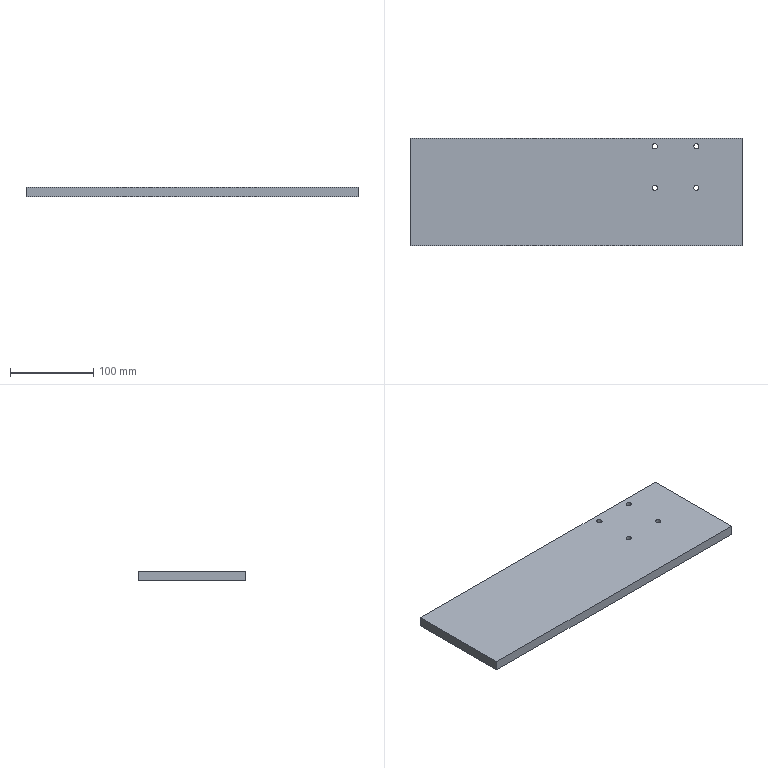Part | SolidWorks | features BaseBody 1 | 1 solid | 14 faces | box 400 x 130 x 12 mm | volume 622504 mm3 | cylinder 8 | plane 6 | commonest cylinder face diameters 6.3 x8
STEP:
#1=CARTESIAN_POINT('',(141.85,55.,-6.));
#2=VERTEX_POINT('',#1);
#3=CARTESIAN_POINT('',(148.15,55.,-6.));
#4=VERTEX_POINT('',#3);
#5=CARTESIAN_POINT('',(145.,55.,-6.));
#6=DIRECTION('',(0.,0.,1.));
#7=DIRECTION('',(1.,0.,0.));
#8=AXIS2_PLACEMENT_3D('',#5,#6,#7);
#9=CIRCLE('',#8,3.15);
#10=EDGE_CURVE('',#2,#4,#9,.T.);
#11=ORIENTED_EDGE('',*,*,#10,.F.);
#12=CARTESIAN_POINT('',(141.85,55.,6.));
#13=VERTEX_POINT('',#12);
#14=CARTESIAN_POINT('',(141.85,55.,-14.2));
#15=DIRECTION('',(0.,0.,1.));
#16=VECTOR('',#15,1000.);
#17=LINE('',#14,#16);
#18=EDGE_CURVE('',#2,#13,#17,.T.);
#19=ORIENTED_EDGE('',*,*,#18,.T.);
#20=CARTESIAN_POINT('',(148.15,55.,6.));
#21=VERTEX_POINT('',#20);
#22=CARTESIAN_POINT('',(145.,55.,6.));
#23=DIRECTION('',(0.,0.,-1.));
#24=DIRECTION('',(1.,0.,0.));
#25=AXIS2_PLACEMENT_3D('',#22,#23,#24);
#26=CIRCLE('',#25,3.15);
#27=EDGE_CURVE('',#21,#13,#26,.T.);
#28=ORIENTED_EDGE('',*,*,#27,.F.);
#29=CARTESIAN_POINT('',(148.15,55.,-14.2));
#30=DIRECTION('',(0.,0.,1.));
#31=VECTOR('',#30,1000.);
#32=LINE('',#29,#31);
#33=EDGE_CURVE('',#4,#21,#32,.T.);
#34=ORIENTED_EDGE('',*,*,#33,.F.);
#35=EDGE_LOOP('',(#11,#19,#28,#34));
#36=FACE_OUTER_BOUND('',#35,.T.);
#37=CARTESIAN_POINT('',(145.,55.,-14.2));
#38=DIRECTION('',(0.,0.,1.));
#39=DIRECTION('',(1.,0.,0.));
#40=AXIS2_PLACEMENT_3D('',#37,#38,#39);
#41=CYLINDRICAL_SURFACE('',#40,3.15);
#42=ADVANCED_FACE('',(#36),#41,.F.);
#43=CARTESIAN_POINT('',(91.85,55.,-6.));
#44=VERTEX_POINT('',#43);
#45=CARTESIAN_POINT('',(98.15,55.,-6.));
#46=VERTEX_POINT('',#45);
#47=CARTESIAN_POINT('',(95.,55.,-6.));
#48=DIRECTION('',(0.,0.,1.));
#49=DIRECTION('',(1.,0.,0.));
#50=AXIS2_PLACEMENT_3D('',#47,#48,#49);
#51=CIRCLE('',#50,3.15);
#52=EDGE_CURVE('',#44,#46,#51,.T.);
#53=ORIENTED_EDGE('',*,*,#52,.F.);
#54=CARTESIAN_POINT('',(91.85,55.,6.));
#55=VERTEX_POINT('',#54);
#56=CARTESIAN_POINT('',(91.85,55.,-14.2));
#57=DIRECTION('',(0.,0.,1.));
#58=VECTOR('',#57,1000.);
#59=LINE('',#56,#58);
#60=EDGE_CURVE('',#44,#55,#59,.T.);
#61=ORIENTED_EDGE('',*,*,#60,.T.);
#62=CARTESIAN_POINT('',(98.15,55.,6.));
#63=VERTEX_POINT('',#62);
#64=CARTESIAN_POINT('',(95.,55.,6.));
#65=DIRECTION('',(0.,0.,-1.));
#66=DIRECTION('',(1.,0.,0.));
#67=AXIS2_PLACEMENT_3D('',#64,#65,#66);
#68=CIRCLE('',#67,3.15);
#69=EDGE_CURVE('',#63,#55,#68,.T.);
#70=ORIENTED_EDGE('',*,*,#69,.F.);
#71=CARTESIAN_POINT('',(98.15,55.,-14.2));
#72=DIRECTION('',(0.,0.,1.));
#73=VECTOR('',#72,1000.);
#74=LINE('',#71,#73);
#75=EDGE_CURVE('',#46,#63,#74,.T.);
#76=ORIENTED_EDGE('',*,*,#75,.F.);
#77=EDGE_LOOP('',(#53,#61,#70,#76));
#78=FACE_OUTER_BOUND('',#77,.T.);
#79=CARTESIAN_POINT('',(95.,55.,-14.2));
#80=DIRECTION('',(0.,0.,1.));
#81=DIRECTION('',(1.,0.,0.));
#82=AXIS2_PLACEMENT_3D('',#79,#80,#81);
#83=CYLINDRICAL_SURFACE('',#82,3.15);
#84=ADVANCED_FACE('',(#78),#83,.F.);
#85=CARTESIAN_POINT('',(141.85,5.,-6.));
#86=VERTEX_POINT('',#85);
#87=CARTESIAN_POINT('',(148.15,5.,-6.));
#88=VERTEX_POINT('',#87);
#89=CARTESIAN_POINT('',(145.,5.,-6.));
#90=DIRECTION('',(0.,0.,1.));
#91=DIRECTION('',(1.,0.,0.));
#92=AXIS2_PLACEMENT_3D('',#89,#90,#91);
#93=CIRCLE('',#92,3.15);
#94=EDGE_CURVE('',#86,#88,#93,.T.);
#95=ORIENTED_EDGE('',*,*,#94,.F.);
#96=CARTESIAN_POINT('',(141.85,5.,6.));
#97=VERTEX_POINT('',#96);
#98=CARTESIAN_POINT('',(141.85,5.,-14.2));
#99=DIRECTION('',(0.,0.,1.));
#100=VECTOR('',#99,1000.);
#101=LINE('',#98,#100);
#102=EDGE_CURVE('',#86,#97,#101,.T.);
#103=ORIENTED_EDGE('',*,*,#102,.T.);
#104=CARTESIAN_POINT('',(148.15,5.,6.));
#105=VERTEX_POINT('',#104);
#106=CARTESIAN_POINT('',(145.,5.,6.));
#107=DIRECTION('',(0.,0.,-1.));
#108=DIRECTION('',(1.,0.,0.));
#109=AXIS2_PLACEMENT_3D('',#106,#107,#108);
#110=CIRCLE('',#109,3.15);
#111=EDGE_CURVE('',#105,#97,#110,.T.);
#112=ORIENTED_EDGE('',*,*,#111,.F.);
#113=CARTESIAN_POINT('',(148.15,5.,-14.2));
#114=DIRECTION('',(0.,0.,1.));
#115=VECTOR('',#114,1000.);
#116=LINE('',#113,#115);
#117=EDGE_CURVE('',#88,#105,#116,.T.);
#118=ORIENTED_EDGE('',*,*,#117,.F.);
#119=EDGE_LOOP('',(#95,#103,#112,#118));
#120=FACE_OUTER_BOUND('',#119,.T.);
#121=CARTESIAN_POINT('',(145.,5.,-14.2));
#122=DIRECTION('',(0.,0.,1.));
#123=DIRECTION('',(1.,0.,0.));
#124=AXIS2_PLACEMENT_3D('',#121,#122,#123);
#125=CYLINDRICAL_SURFACE('',#124,3.15);
#126=ADVANCED_FACE('',(#120),#125,.F.);
#127=CARTESIAN_POINT('',(91.85,5.,-6.));
#128=VERTEX_POINT('',#127);
#129=CARTESIAN_POINT('',(98.15,5.,-6.));
#130=VERTEX_POINT('',#129);
#131=CARTESIAN_POINT('',(95.,5.,-6.));
#132=DIRECTION('',(0.,0.,1.));
#133=DIRECTION('',(1.,0.,0.));
#134=AXIS2_PLACEMENT_3D('',#131,#132,#133);
#135=CIRCLE('',#134,3.15);
#136=EDGE_CURVE('',#128,#130,#135,.T.);
#137=ORIENTED_EDGE('',*,*,#136,.F.);
#138=CARTESIAN_POINT('',(91.85,5.,6.));
#139=VERTEX_POINT('',#138);
#140=CARTESIAN_POINT('',(91.85,5.,-14.2));
#141=DIRECTION('',(0.,0.,1.));
#142=VECTOR('',#141,1000.);
#143=LINE('',#140,#142);
#144=EDGE_CURVE('',#128,#139,#143,.T.);
#145=ORIENTED_EDGE('',*,*,#144,.T.);
#146=CARTESIAN_POINT('',(98.15,5.,6.));
#147=VERTEX_POINT('',#146);
#148=CARTESIAN_POINT('',(95.,5.,6.));
#149=DIRECTION('',(0.,0.,-1.));
#150=DIRECTION('',(1.,0.,0.));
#151=AXIS2_PLACEMENT_3D('',#148,#149,#150);
#152=CIRCLE('',#151,3.15);
#153=EDGE_CURVE('',#147,#139,#152,.T.);
#154=ORIENTED_EDGE('',*,*,#153,.F.);
#155=CARTESIAN_POINT('',(98.15,5.,-14.2));
#156=DIRECTION('',(0.,0.,1.));
#157=VECTOR('',#156,1000.);
#158=LINE('',#155,#157);
#159=EDGE_CURVE('',#130,#147,#158,.T.);
#160=ORIENTED_EDGE('',*,*,#159,.F.);
#161=EDGE_LOOP('',(#137,#145,#154,#160));
#162=FACE_OUTER_BOUND('',#161,.T.);
#163=CARTESIAN_POINT('',(95.,5.,-14.2));
#164=DIRECTION('',(0.,0.,1.));
#165=DIRECTION('',(1.,0.,0.));
#166=AXIS2_PLACEMENT_3D('',#163,#164,#165);
#167=CYLINDRICAL_SURFACE('',#166,3.15);
#168=ADVANCED_FACE('',(#162),#167,.F.);
#169=ORIENTED_EDGE('',*,*,#27,.T.);
#170=CARTESIAN_POINT('',(145.,55.,6.));
#171=DIRECTION('',(0.,0.,-1.));
#172=DIRECTION('',(1.,0.,0.));
#173=AXIS2_PLACEMENT_3D('',#170,#171,#172);
#174=CIRCLE('',#173,3.15);
#175=EDGE_CURVE('',#13,#21,#174,.T.);
#176=ORIENTED_EDGE('',*,*,#175,.T.);
#177=EDGE_LOOP('',(#169,#176));
#178=FACE_BOUND('',#177,.T.);
#179=ORIENTED_EDGE('',*,*,#69,.T.);
#180=CARTESIAN_POINT('',(95.,55.,6.));
#181=DIRECTION('',(0.,0.,-1.));
#182=DIRECTION('',(1.,0.,0.));
#183=AXIS2_PLACEMENT_3D('',#180,#181,#182);
#184=CIRCLE('',#183,3.15);
#185=EDGE_CURVE('',#55,#63,#184,.T.);
#186=ORIENTED_EDGE('',*,*,#185,.T.);
#187=EDGE_LOOP('',(#179,#186));
#188=FACE_BOUND('',#187,.T.);
#189=ORIENTED_EDGE('',*,*,#111,.T.);
#190=CARTESIAN_POINT('',(145.,5.,6.));
#191=DIRECTION('',(0.,0.,-1.));
#192=DIRECTION('',(1.,0.,0.));
#193=AXIS2_PLACEMENT_3D('',#190,#191,#192);
#194=CIRCLE('',#193,3.15);
#195=EDGE_CURVE('',#97,#105,#194,.T.);
#196=ORIENTED_EDGE('',*,*,#195,.T.);
#197=EDGE_LOOP('',(#189,#196));
#198=FACE_BOUND('',#197,.T.);
#199=ORIENTED_EDGE('',*,*,#153,.T.);
#200=CARTESIAN_POINT('',(95.,5.,6.));
#201=DIRECTION('',(0.,0.,-1.));
#202=DIRECTION('',(1.,0.,0.));
#203=AXIS2_PLACEMENT_3D('',#200,#201,#202);
#204=CIRCLE('',#203,3.15);
#205=EDGE_CURVE('',#139,#147,#204,.T.);
#206=ORIENTED_EDGE('',*,*,#205,.T.);
#207=EDGE_LOOP('',(#199,#206));
#208=FACE_BOUND('',#207,.T.);
#209=CARTESIAN_POINT('',(200.,-65.,6.));
#210=VERTEX_POINT('',#209);
#211=CARTESIAN_POINT('',(200.,65.,6.));
#212=VERTEX_POINT('',#211);
#213=CARTESIAN_POINT('',(200.,-65.,6.));
#214=DIRECTION('',(0.,1.,0.));
#215=VECTOR('',#214,1000.);
#216=LINE('',#213,#215);
#217=EDGE_CURVE('',#210,#212,#216,.T.);
#218=ORIENTED_EDGE('',*,*,#217,.T.);
#219=CARTESIAN_POINT('',(-200.,65.,6.));
#220=VERTEX_POINT('',#219);
#221=CARTESIAN_POINT('',(-200.,65.,6.));
#222=DIRECTION('',(-1.,0.,0.));
#223=VECTOR('',#222,1000.);
#224=LINE('',#221,#223);
#225=EDGE_CURVE('',#212,#220,#224,.T.);
#226=ORIENTED_EDGE('',*,*,#225,.T.);
#227=CARTESIAN_POINT('',(-200.,-65.,6.));
#228=VERTEX_POINT('',#227);
#229=CARTESIAN_POINT('',(-200.,-65.,6.));
#230=DIRECTION('',(0.,-1.,0.));
#231=VECTOR('',#230,1000.);
#232=LINE('',#229,#231);
#233=EDGE_CURVE('',#220,#228,#232,.T.);
#234=ORIENTED_EDGE('',*,*,#233,.T.);
#235=CARTESIAN_POINT('',(-200.,-65.,6.));
#236=DIRECTION('',(1.,0.,0.));
#237=VECTOR('',#236,1000.);
#238=LINE('',#235,#237);
#239=EDGE_CURVE('',#228,#210,#238,.T.);
#240=ORIENTED_EDGE('',*,*,#239,.T.);
#241=EDGE_LOOP('',(#218,#226,#234,#240));
#242=FACE_OUTER_BOUND('',#241,.T.);
#243=CARTESIAN_POINT('',(-200.,-65.,6.));
#244=DIRECTION('',(0.,0.,1.));
#245=DIRECTION('',(1.,0.,0.));
#246=AXIS2_PLACEMENT_3D('',#243,#244,#245);
#247=PLANE('',#246);
#248=ADVANCED_FACE('',(#178,#188,#198,#208,#242),#247,.T.);
#249=ORIENTED_EDGE('',*,*,#18,.F.);
#250=CARTESIAN_POINT('',(145.,55.,-6.));
#251=DIRECTION('',(0.,0.,1.));
#252=DIRECTION('',(1.,0.,0.));
#253=AXIS2_PLACEMENT_3D('',#250,#251,#252);
#254=CIRCLE('',#253,3.15);
#255=EDGE_CURVE('',#4,#2,#254,.T.);
#256=ORIENTED_EDGE('',*,*,#255,.F.);
#257=ORIENTED_EDGE('',*,*,#33,.T.);
#258=ORIENTED_EDGE('',*,*,#175,.F.);
#259=EDGE_LOOP('',(#249,#256,#257,#258));
#260=FACE_OUTER_BOUND('',#259,.T.);
#261=CARTESIAN_POINT('',(145.,55.,-14.2));
#262=DIRECTION('',(0.,0.,1.));
#263=DIRECTION('',(1.,0.,0.));
#264=AXIS2_PLACEMENT_3D('',#261,#262,#263);
#265=CYLINDRICAL_SURFACE('',#264,3.15);
#266=ADVANCED_FACE('',(#260),#265,.F.);
#267=ORIENTED_EDGE('',*,*,#60,.F.);
#268=CARTESIAN_POINT('',(95.,55.,-6.));
#269=DIRECTION('',(0.,0.,1.));
#270=DIRECTION('',(1.,0.,0.));
#271=AXIS2_PLACEMENT_3D('',#268,#269,#270);
#272=CIRCLE('',#271,3.15);
#273=EDGE_CURVE('',#46,#44,#272,.T.);
#274=ORIENTED_EDGE('',*,*,#273,.F.);
#275=ORIENTED_EDGE('',*,*,#75,.T.);
#276=ORIENTED_EDGE('',*,*,#185,.F.);
#277=EDGE_LOOP('',(#267,#274,#275,#276));
#278=FACE_OUTER_BOUND('',#277,.T.);
#279=CARTESIAN_POINT('',(95.,55.,-14.2));
#280=DIRECTION('',(0.,0.,1.));
#281=DIRECTION('',(1.,0.,0.));
#282=AXIS2_PLACEMENT_3D('',#279,#280,#281);
#283=CYLINDRICAL_SURFACE('',#282,3.15);
#284=ADVANCED_FACE('',(#278),#283,.F.);
#285=ORIENTED_EDGE('',*,*,#102,.F.);
#286=CARTESIAN_POINT('',(145.,5.,-6.));
#287=DIRECTION('',(0.,0.,1.));
#288=DIRECTION('',(1.,0.,0.));
#289=AXIS2_PLACEMENT_3D('',#286,#287,#288);
#290=CIRCLE('',#289,3.15);
#291=EDGE_CURVE('',#88,#86,#290,.T.);
#292=ORIENTED_EDGE('',*,*,#291,.F.);
#293=ORIENTED_EDGE('',*,*,#117,.T.);
#294=ORIENTED_EDGE('',*,*,#195,.F.);
#295=EDGE_LOOP('',(#285,#292,#293,#294));
#296=FACE_OUTER_BOUND('',#295,.T.);
#297=CARTESIAN_POINT('',(145.,5.,-14.2));
#298=DIRECTION('',(0.,0.,1.));
#299=DIRECTION('',(1.,0.,0.));
#300=AXIS2_PLACEMENT_3D('',#297,#298,#299);
#301=CYLINDRICAL_SURFACE('',#300,3.15);
#302=ADVANCED_FACE('',(#296),#301,.F.);
#303=ORIENTED_EDGE('',*,*,#144,.F.);
#304=CARTESIAN_POINT('',(95.,5.,-6.));
#305=DIRECTION('',(0.,0.,1.));
#306=DIRECTION('',(1.,0.,0.));
#307=AXIS2_PLACEMENT_3D('',#304,#305,#306);
#308=CIRCLE('',#307,3.15);
#309=EDGE_CURVE('',#130,#128,#308,.T.);
#310=ORIENTED_EDGE('',*,*,#309,.F.);
#311=ORIENTED_EDGE('',*,*,#159,.T.);
#312=ORIENTED_EDGE('',*,*,#205,.F.);
#313=EDGE_LOOP('',(#303,#310,#311,#312));
#314=FACE_OUTER_BOUND('',#313,.T.);
#315=CARTESIAN_POINT('',(95.,5.,-14.2));
#316=DIRECTION('',(0.,0.,1.));
#317=DIRECTION('',(1.,0.,0.));
#318=AXIS2_PLACEMENT_3D('',#315,#316,#317);
#319=CYLINDRICAL_SURFACE('',#318,3.15);
#320=ADVANCED_FACE('',(#314),#319,.F.);
#321=ORIENTED_EDGE('',*,*,#225,.F.);
#322=CARTESIAN_POINT('',(200.,65.,-6.));
#323=VERTEX_POINT('',#322);
#324=CARTESIAN_POINT('',(200.,65.,-6.));
#325=DIRECTION('',(0.,0.,-1.));
#326=VECTOR('',#325,1000.);
#327=LINE('',#324,#326);
#328=EDGE_CURVE('',#212,#323,#327,.T.);
#329=ORIENTED_EDGE('',*,*,#328,.T.);
#330=CARTESIAN_POINT('',(-200.,65.,-6.));
#331=VERTEX_POINT('',#330);
#332=CARTESIAN_POINT('',(-200.,65.,-6.));
#333=DIRECTION('',(-1.,0.,0.));
#334=VECTOR('',#333,1000.);
#335=LINE('',#332,#334);
#336=EDGE_CURVE('',#323,#331,#335,.T.);
#337=ORIENTED_EDGE('',*,*,#336,.T.);
#338=CARTESIAN_POINT('',(-200.,65.,-6.));
#339=DIRECTION('',(0.,0.,1.));
#340=VECTOR('',#339,1000.);
#341=LINE('',#338,#340);
#342=EDGE_CURVE('',#331,#220,#341,.T.);
#343=ORIENTED_EDGE('',*,*,#342,.T.);
#344=EDGE_LOOP('',(#321,#329,#337,#343));
#345=FACE_OUTER_BOUND('',#344,.T.);
#346=CARTESIAN_POINT('',(-200.,65.,-6.));
#347=DIRECTION('',(0.,1.,0.));
#348=DIRECTION('',(0.,0.,1.));
#349=AXIS2_PLACEMENT_3D('',#346,#347,#348);
#350=PLANE('',#349);
#351=ADVANCED_FACE('',(#345),#350,.T.);
#352=ORIENTED_EDGE('',*,*,#328,.F.);
#353=ORIENTED_EDGE('',*,*,#217,.F.);
#354=CARTESIAN_POINT('',(200.,-65.,-6.));
#355=VERTEX_POINT('',#354);
#356=CARTESIAN_POINT('',(200.,-65.,-6.));
#357=DIRECTION('',(0.,0.,-1.));
#358=VECTOR('',#357,1000.);
#359=LINE('',#356,#358);
#360=EDGE_CURVE('',#210,#355,#359,.T.);
#361=ORIENTED_EDGE('',*,*,#360,.T.);
#362=CARTESIAN_POINT('',(200.,-65.,-6.));
#363=DIRECTION('',(0.,1.,0.));
#364=VECTOR('',#363,1000.);
#365=LINE('',#362,#364);
#366=EDGE_CURVE('',#355,#323,#365,.T.);
#367=ORIENTED_EDGE('',*,*,#366,.T.);
#368=EDGE_LOOP('',(#352,#353,#361,#367));
#369=FACE_OUTER_BOUND('',#368,.T.);
#370=CARTESIAN_POINT('',(200.,-65.,-6.));
#371=DIRECTION('',(1.,0.,0.));
#372=DIRECTION('',(0.,0.,-1.));
#373=AXIS2_PLACEMENT_3D('',#370,#371,#372);
#374=PLANE('',#373);
#375=ADVANCED_FACE('',(#369),#374,.T.);
#376=ORIENTED_EDGE('',*,*,#239,.F.);
#377=CARTESIAN_POINT('',(-200.,-65.,-6.));
#378=VERTEX_POINT('',#377);
#379=CARTESIAN_POINT('',(-200.,-65.,-6.));
#380=DIRECTION('',(0.,0.,1.));
#381=VECTOR('',#380,1000.);
#382=LINE('',#379,#381);
#383=EDGE_CURVE('',#378,#228,#382,.T.);
#384=ORIENTED_EDGE('',*,*,#383,.F.);
#385=CARTESIAN_POINT('',(-200.,-65.,-6.));
#386=DIRECTION('',(-1.,0.,0.));
#387=VECTOR('',#386,1000.);
#388=LINE('',#385,#387);
#389=EDGE_CURVE('',#355,#378,#388,.T.);
#390=ORIENTED_EDGE('',*,*,#389,.F.);
#391=ORIENTED_EDGE('',*,*,#360,.F.);
#392=EDGE_LOOP('',(#376,#384,#390,#391));
#393=FACE_OUTER_BOUND('',#392,.T.);
#394=CARTESIAN_POINT('',(-200.,-65.,-6.));
#395=DIRECTION('',(0.,1.,0.));
#396=DIRECTION('',(0.,0.,1.));
#397=AXIS2_PLACEMENT_3D('',#394,#395,#396);
#398=PLANE('',#397);
#399=ADVANCED_FACE('',(#393),#398,.F.);
#400=ORIENTED_EDGE('',*,*,#342,.F.);
#401=CARTESIAN_POINT('',(-200.,-65.,-6.));
#402=DIRECTION('',(0.,1.,0.));
#403=VECTOR('',#402,1000.);
#404=LINE('',#401,#403);
#405=EDGE_CURVE('',#378,#331,#404,.T.);
#406=ORIENTED_EDGE('',*,*,#405,.F.);
#407=ORIENTED_EDGE('',*,*,#383,.T.);
#408=ORIENTED_EDGE('',*,*,#233,.F.);
#409=EDGE_LOOP('',(#400,#406,#407,#408));
#410=FACE_OUTER_BOUND('',#409,.T.);
#411=CARTESIAN_POINT('',(-200.,-65.,-6.));
#412=DIRECTION('',(1.,0.,0.));
#413=DIRECTION('',(0.,0.,-1.));
#414=AXIS2_PLACEMENT_3D('',#411,#412,#413);
#415=PLANE('',#414);
#416=ADVANCED_FACE('',(#410),#415,.F.);
#417=ORIENTED_EDGE('',*,*,#255,.T.);
#418=ORIENTED_EDGE('',*,*,#10,.T.);
#419=EDGE_LOOP('',(#417,#418));
#420=FACE_BOUND('',#419,.T.);
#421=ORIENTED_EDGE('',*,*,#273,.T.);
#422=ORIENTED_EDGE('',*,*,#52,.T.);
#423=EDGE_LOOP('',(#421,#422));
#424=FACE_BOUND('',#423,.T.);
#425=ORIENTED_EDGE('',*,*,#291,.T.);
#426=ORIENTED_EDGE('',*,*,#94,.T.);
#427=EDGE_LOOP('',(#425,#426));
#428=FACE_BOUND('',#427,.T.);
#429=ORIENTED_EDGE('',*,*,#309,.T.);
#430=ORIENTED_EDGE('',*,*,#136,.T.);
#431=EDGE_LOOP('',(#429,#430));
#432=FACE_BOUND('',#431,.T.);
#433=ORIENTED_EDGE('',*,*,#366,.F.);
#434=ORIENTED_EDGE('',*,*,#389,.T.);
#435=ORIENTED_EDGE('',*,*,#405,.T.);
#436=ORIENTED_EDGE('',*,*,#336,.F.);
#437=EDGE_LOOP('',(#433,#434,#435,#436));
#438=FACE_OUTER_BOUND('',#437,.T.);
#439=CARTESIAN_POINT('',(-200.,-65.,-6.));
#440=DIRECTION('',(0.,0.,1.));
#441=DIRECTION('',(1.,0.,0.));
#442=AXIS2_PLACEMENT_3D('',#439,#440,#441);
#443=PLANE('',#442);
#444=ADVANCED_FACE('',(#420,#424,#428,#432,#438),#443,.F.);
#445=CLOSED_SHELL('',(#42,#84,#126,#168,#248,#266,#284,#302,#320,#351,#375,#399,#416,#444));
#446=MANIFOLD_SOLID_BREP('',#445);
#447=CARTESIAN_POINT('',(0.,0.,0.));
#448=DIRECTION('',(0.,0.,1.));
#449=DIRECTION('',(1.,0.,0.));
#450=AXIS2_PLACEMENT_3D('',#447,#448,#449);
#451=(LENGTH_UNIT()NAMED_UNIT(*)SI_UNIT(.MILLI.,.METRE.));
#452=UNCERTAINTY_MEASURE_WITH_UNIT(LENGTH_MEASURE(0.00001),#451,'','');
#453=(NAMED_UNIT(*)PLANE_ANGLE_UNIT()SI_UNIT($,.RADIAN.));
#454=(NAMED_UNIT(*)SI_UNIT($,.STERADIAN.)SOLID_ANGLE_UNIT());
#455=(GEOMETRIC_REPRESENTATION_CONTEXT(3)GLOBAL_UNCERTAINTY_ASSIGNED_CONTEXT((#452))GLOBAL_UNIT_ASSIGNED_CONTEXT((#451,#453,#454))REPRESENTATION_CONTEXT('',''));
#456=ADVANCED_BREP_SHAPE_REPRESENTATION('',(#446,#450),#455);